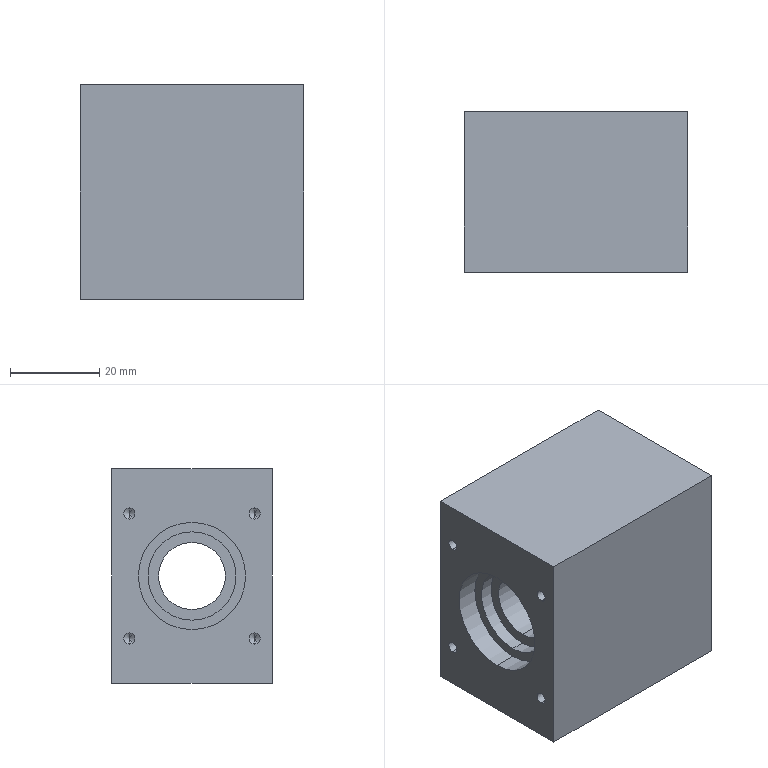Part | SolidWorks | features ICE 3, HoleWzd 2, Extrusion 1, MirrorPattern 1 | 1 solid | 56 faces | box 50 x 36 x 48 mm | volume 72690 mm3 | cylinder 30 | cone 16 | plane 10 | commonest cylinder face diameters 2.5 x8 4.2 x8 4 x4 19.8 x4 24 x4 15 x2